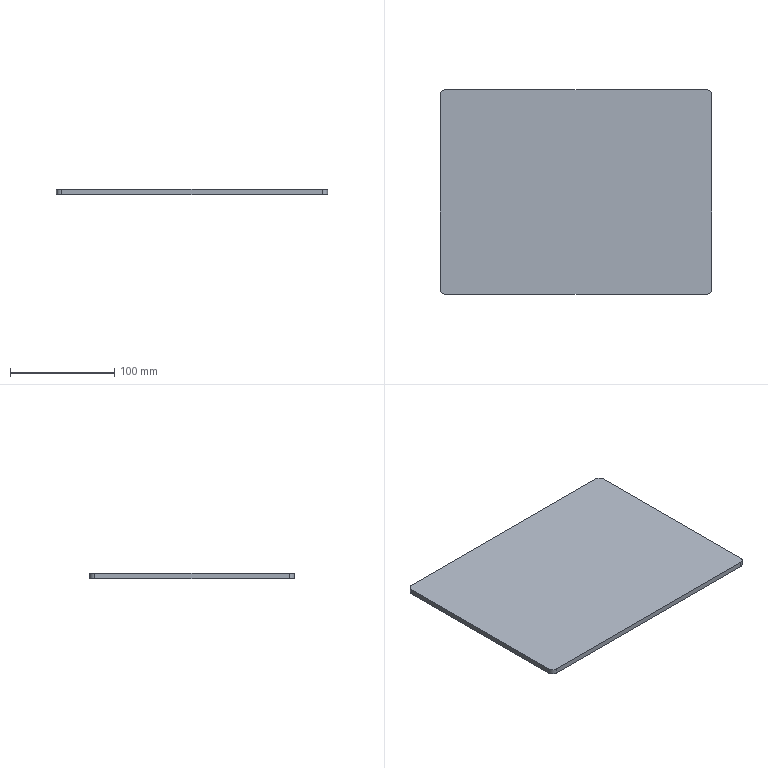Part | SolidWorks | features Extrusion 1, Fillet 1 | 1 solid | 10 faces | box 260 x 196 x 5 mm | volume 254693 mm3 | plane 6 | cylinder 4 | commonest cylinder face diameters 10 x4
STEP:
#1=CARTESIAN_POINT('',(0.,-5.,0.));
#2=VERTEX_POINT('',#1);
#3=CARTESIAN_POINT('',(0.,-191.,0.));
#4=VERTEX_POINT('',#3);
#5=CARTESIAN_POINT('',(0.,0.,0.));
#6=DIRECTION('',(0.,-1.,0.));
#7=VECTOR('',#6,1000.);
#8=LINE('',#5,#7);
#9=EDGE_CURVE('',#2,#4,#8,.T.);
#10=ORIENTED_EDGE('',*,*,#9,.T.);
#11=CARTESIAN_POINT('',(0.,-191.,5.));
#12=VERTEX_POINT('',#11);
#13=CARTESIAN_POINT('',(0.,-191.,5.));
#14=DIRECTION('',(0.,0.,1.));
#15=VECTOR('',#14,1000.);
#16=LINE('',#13,#15);
#17=EDGE_CURVE('',#4,#12,#16,.T.);
#18=ORIENTED_EDGE('',*,*,#17,.T.);
#19=CARTESIAN_POINT('',(0.,-5.,5.));
#20=VERTEX_POINT('',#19);
#21=CARTESIAN_POINT('',(0.,0.,5.));
#22=DIRECTION('',(0.,-1.,0.));
#23=VECTOR('',#22,1000.);
#24=LINE('',#21,#23);
#25=EDGE_CURVE('',#20,#12,#24,.T.);
#26=ORIENTED_EDGE('',*,*,#25,.F.);
#27=CARTESIAN_POINT('',(0.,-5.,5.));
#28=DIRECTION('',(0.,0.,-1.));
#29=VECTOR('',#28,1000.);
#30=LINE('',#27,#29);
#31=EDGE_CURVE('',#20,#2,#30,.T.);
#32=ORIENTED_EDGE('',*,*,#31,.T.);
#33=EDGE_LOOP('',(#10,#18,#26,#32));
#34=FACE_OUTER_BOUND('',#33,.T.);
#35=CARTESIAN_POINT('',(0.,0.,5.));
#36=DIRECTION('',(1.,0.,0.));
#37=DIRECTION('',(0.,1.,0.));
#38=AXIS2_PLACEMENT_3D('',#35,#36,#37);
#39=PLANE('',#38);
#40=ADVANCED_FACE('',(#34),#39,.F.);
#41=CARTESIAN_POINT('',(5.,-196.,0.));
#42=VERTEX_POINT('',#41);
#43=CARTESIAN_POINT('',(255.,-196.,0.));
#44=VERTEX_POINT('',#43);
#45=CARTESIAN_POINT('',(0.,-196.,0.));
#46=DIRECTION('',(1.,0.,0.));
#47=VECTOR('',#46,1000.);
#48=LINE('',#45,#47);
#49=EDGE_CURVE('',#42,#44,#48,.T.);
#50=ORIENTED_EDGE('',*,*,#49,.T.);
#51=CARTESIAN_POINT('',(255.,-196.,5.));
#52=VERTEX_POINT('',#51);
#53=CARTESIAN_POINT('',(255.,-196.,5.));
#54=DIRECTION('',(0.,0.,1.));
#55=VECTOR('',#54,1000.);
#56=LINE('',#53,#55);
#57=EDGE_CURVE('',#44,#52,#56,.T.);
#58=ORIENTED_EDGE('',*,*,#57,.T.);
#59=CARTESIAN_POINT('',(5.,-196.,5.));
#60=VERTEX_POINT('',#59);
#61=CARTESIAN_POINT('',(0.,-196.,5.));
#62=DIRECTION('',(1.,0.,0.));
#63=VECTOR('',#62,1000.);
#64=LINE('',#61,#63);
#65=EDGE_CURVE('',#60,#52,#64,.T.);
#66=ORIENTED_EDGE('',*,*,#65,.F.);
#67=CARTESIAN_POINT('',(5.,-196.,5.));
#68=DIRECTION('',(0.,0.,-1.));
#69=VECTOR('',#68,1000.);
#70=LINE('',#67,#69);
#71=EDGE_CURVE('',#60,#42,#70,.T.);
#72=ORIENTED_EDGE('',*,*,#71,.T.);
#73=EDGE_LOOP('',(#50,#58,#66,#72));
#74=FACE_OUTER_BOUND('',#73,.T.);
#75=CARTESIAN_POINT('',(0.,-196.,5.));
#76=DIRECTION('',(0.,1.,0.));
#77=DIRECTION('',(0.,0.,1.));
#78=AXIS2_PLACEMENT_3D('',#75,#76,#77);
#79=PLANE('',#78);
#80=ADVANCED_FACE('',(#74),#79,.F.);
#81=CARTESIAN_POINT('',(260.,-191.,0.));
#82=VERTEX_POINT('',#81);
#83=CARTESIAN_POINT('',(260.,-5.,0.));
#84=VERTEX_POINT('',#83);
#85=CARTESIAN_POINT('',(260.,0.,0.));
#86=DIRECTION('',(0.,1.,0.));
#87=VECTOR('',#86,1000.);
#88=LINE('',#85,#87);
#89=EDGE_CURVE('',#82,#84,#88,.T.);
#90=ORIENTED_EDGE('',*,*,#89,.T.);
#91=CARTESIAN_POINT('',(260.,-5.,5.));
#92=VERTEX_POINT('',#91);
#93=CARTESIAN_POINT('',(260.,-5.,5.));
#94=DIRECTION('',(0.,0.,1.));
#95=VECTOR('',#94,1000.);
#96=LINE('',#93,#95);
#97=EDGE_CURVE('',#84,#92,#96,.T.);
#98=ORIENTED_EDGE('',*,*,#97,.T.);
#99=CARTESIAN_POINT('',(260.,-191.,5.));
#100=VERTEX_POINT('',#99);
#101=CARTESIAN_POINT('',(260.,0.,5.));
#102=DIRECTION('',(0.,1.,0.));
#103=VECTOR('',#102,1000.);
#104=LINE('',#101,#103);
#105=EDGE_CURVE('',#100,#92,#104,.T.);
#106=ORIENTED_EDGE('',*,*,#105,.F.);
#107=CARTESIAN_POINT('',(260.,-191.,5.));
#108=DIRECTION('',(0.,0.,-1.));
#109=VECTOR('',#108,1000.);
#110=LINE('',#107,#109);
#111=EDGE_CURVE('',#100,#82,#110,.T.);
#112=ORIENTED_EDGE('',*,*,#111,.T.);
#113=EDGE_LOOP('',(#90,#98,#106,#112));
#114=FACE_OUTER_BOUND('',#113,.T.);
#115=CARTESIAN_POINT('',(260.,0.,5.));
#116=DIRECTION('',(-1.,0.,0.));
#117=DIRECTION('',(0.,0.,1.));
#118=AXIS2_PLACEMENT_3D('',#115,#116,#117);
#119=PLANE('',#118);
#120=ADVANCED_FACE('',(#114),#119,.F.);
#121=CARTESIAN_POINT('',(255.,0.,5.));
#122=VERTEX_POINT('',#121);
#123=CARTESIAN_POINT('',(5.,0.,5.));
#124=VERTEX_POINT('',#123);
#125=CARTESIAN_POINT('',(0.,0.,5.));
#126=DIRECTION('',(-1.,0.,0.));
#127=VECTOR('',#126,1000.);
#128=LINE('',#125,#127);
#129=EDGE_CURVE('',#122,#124,#128,.T.);
#130=ORIENTED_EDGE('',*,*,#129,.F.);
#131=CARTESIAN_POINT('',(255.,0.,0.));
#132=VERTEX_POINT('',#131);
#133=CARTESIAN_POINT('',(255.,0.,5.));
#134=DIRECTION('',(0.,0.,-1.));
#135=VECTOR('',#134,1000.);
#136=LINE('',#133,#135);
#137=EDGE_CURVE('',#122,#132,#136,.T.);
#138=ORIENTED_EDGE('',*,*,#137,.T.);
#139=CARTESIAN_POINT('',(5.,0.,0.));
#140=VERTEX_POINT('',#139);
#141=CARTESIAN_POINT('',(0.,0.,0.));
#142=DIRECTION('',(-1.,0.,0.));
#143=VECTOR('',#142,1000.);
#144=LINE('',#141,#143);
#145=EDGE_CURVE('',#132,#140,#144,.T.);
#146=ORIENTED_EDGE('',*,*,#145,.T.);
#147=CARTESIAN_POINT('',(5.,0.,5.));
#148=DIRECTION('',(0.,0.,1.));
#149=VECTOR('',#148,1000.);
#150=LINE('',#147,#149);
#151=EDGE_CURVE('',#140,#124,#150,.T.);
#152=ORIENTED_EDGE('',*,*,#151,.T.);
#153=EDGE_LOOP('',(#130,#138,#146,#152));
#154=FACE_OUTER_BOUND('',#153,.T.);
#155=CARTESIAN_POINT('',(0.,0.,5.));
#156=DIRECTION('',(0.,-1.,0.));
#157=DIRECTION('',(0.,0.,-1.));
#158=AXIS2_PLACEMENT_3D('',#155,#156,#157);
#159=PLANE('',#158);
#160=ADVANCED_FACE('',(#154),#159,.F.);
#161=ORIENTED_EDGE('',*,*,#105,.T.);
#162=CARTESIAN_POINT('',(255.,-5.,5.));
#163=DIRECTION('',(0.,0.,1.));
#164=DIRECTION('',(1.,0.,0.));
#165=AXIS2_PLACEMENT_3D('',#162,#163,#164);
#166=CIRCLE('',#165,5.);
#167=EDGE_CURVE('',#92,#122,#166,.T.);
#168=ORIENTED_EDGE('',*,*,#167,.T.);
#169=ORIENTED_EDGE('',*,*,#129,.T.);
#170=CARTESIAN_POINT('',(5.,-5.,5.));
#171=DIRECTION('',(0.,0.,1.));
#172=DIRECTION('',(1.,0.,0.));
#173=AXIS2_PLACEMENT_3D('',#170,#171,#172);
#174=CIRCLE('',#173,5.);
#175=EDGE_CURVE('',#124,#20,#174,.T.);
#176=ORIENTED_EDGE('',*,*,#175,.T.);
#177=ORIENTED_EDGE('',*,*,#25,.T.);
#178=CARTESIAN_POINT('',(5.,-191.,5.));
#179=DIRECTION('',(0.,0.,1.));
#180=DIRECTION('',(1.,0.,0.));
#181=AXIS2_PLACEMENT_3D('',#178,#179,#180);
#182=CIRCLE('',#181,5.);
#183=EDGE_CURVE('',#12,#60,#182,.T.);
#184=ORIENTED_EDGE('',*,*,#183,.T.);
#185=ORIENTED_EDGE('',*,*,#65,.T.);
#186=CARTESIAN_POINT('',(255.,-191.,5.));
#187=DIRECTION('',(0.,0.,1.));
#188=DIRECTION('',(1.,0.,0.));
#189=AXIS2_PLACEMENT_3D('',#186,#187,#188);
#190=CIRCLE('',#189,5.);
#191=EDGE_CURVE('',#52,#100,#190,.T.);
#192=ORIENTED_EDGE('',*,*,#191,.T.);
#193=EDGE_LOOP('',(#161,#168,#169,#176,#177,#184,#185,#192));
#194=FACE_OUTER_BOUND('',#193,.T.);
#195=CARTESIAN_POINT('',(0.,0.,5.));
#196=DIRECTION('',(0.,0.,1.));
#197=DIRECTION('',(1.,0.,0.));
#198=AXIS2_PLACEMENT_3D('',#195,#196,#197);
#199=PLANE('',#198);
#200=ADVANCED_FACE('',(#194),#199,.T.);
#201=ORIENTED_EDGE('',*,*,#145,.F.);
#202=CARTESIAN_POINT('',(255.,-5.,0.));
#203=DIRECTION('',(0.,0.,-1.));
#204=DIRECTION('',(1.,0.,0.));
#205=AXIS2_PLACEMENT_3D('',#202,#203,#204);
#206=CIRCLE('',#205,5.);
#207=EDGE_CURVE('',#132,#84,#206,.T.);
#208=ORIENTED_EDGE('',*,*,#207,.T.);
#209=ORIENTED_EDGE('',*,*,#89,.F.);
#210=CARTESIAN_POINT('',(255.,-191.,0.));
#211=DIRECTION('',(0.,0.,-1.));
#212=DIRECTION('',(1.,0.,0.));
#213=AXIS2_PLACEMENT_3D('',#210,#211,#212);
#214=CIRCLE('',#213,5.);
#215=EDGE_CURVE('',#82,#44,#214,.T.);
#216=ORIENTED_EDGE('',*,*,#215,.T.);
#217=ORIENTED_EDGE('',*,*,#49,.F.);
#218=CARTESIAN_POINT('',(5.,-191.,0.));
#219=DIRECTION('',(0.,0.,-1.));
#220=DIRECTION('',(1.,0.,0.));
#221=AXIS2_PLACEMENT_3D('',#218,#219,#220);
#222=CIRCLE('',#221,5.);
#223=EDGE_CURVE('',#42,#4,#222,.T.);
#224=ORIENTED_EDGE('',*,*,#223,.T.);
#225=ORIENTED_EDGE('',*,*,#9,.F.);
#226=CARTESIAN_POINT('',(5.,-5.,0.));
#227=DIRECTION('',(0.,0.,-1.));
#228=DIRECTION('',(1.,0.,0.));
#229=AXIS2_PLACEMENT_3D('',#226,#227,#228);
#230=CIRCLE('',#229,5.);
#231=EDGE_CURVE('',#2,#140,#230,.T.);
#232=ORIENTED_EDGE('',*,*,#231,.T.);
#233=EDGE_LOOP('',(#201,#208,#209,#216,#217,#224,#225,#232));
#234=FACE_OUTER_BOUND('',#233,.T.);
#235=CARTESIAN_POINT('',(0.,0.,0.));
#236=DIRECTION('',(0.,0.,1.));
#237=DIRECTION('',(1.,0.,0.));
#238=AXIS2_PLACEMENT_3D('',#235,#236,#237);
#239=PLANE('',#238);
#240=ADVANCED_FACE('',(#234),#239,.F.);
#241=ORIENTED_EDGE('',*,*,#167,.F.);
#242=ORIENTED_EDGE('',*,*,#97,.F.);
#243=ORIENTED_EDGE('',*,*,#207,.F.);
#244=ORIENTED_EDGE('',*,*,#137,.F.);
#245=EDGE_LOOP('',(#241,#242,#243,#244));
#246=FACE_OUTER_BOUND('',#245,.T.);
#247=CARTESIAN_POINT('',(255.,-5.,5.));
#248=DIRECTION('',(0.,0.,-1.));
#249=DIRECTION('',(-1.,0.,0.));
#250=AXIS2_PLACEMENT_3D('',#247,#248,#249);
#251=CYLINDRICAL_SURFACE('',#250,5.);
#252=ADVANCED_FACE('',(#246),#251,.T.);
#253=ORIENTED_EDGE('',*,*,#191,.F.);
#254=ORIENTED_EDGE('',*,*,#57,.F.);
#255=ORIENTED_EDGE('',*,*,#215,.F.);
#256=ORIENTED_EDGE('',*,*,#111,.F.);
#257=EDGE_LOOP('',(#253,#254,#255,#256));
#258=FACE_OUTER_BOUND('',#257,.T.);
#259=CARTESIAN_POINT('',(255.,-191.,5.));
#260=DIRECTION('',(0.,0.,-1.));
#261=DIRECTION('',(-1.,0.,0.));
#262=AXIS2_PLACEMENT_3D('',#259,#260,#261);
#263=CYLINDRICAL_SURFACE('',#262,5.);
#264=ADVANCED_FACE('',(#258),#263,.T.);
#265=ORIENTED_EDGE('',*,*,#183,.F.);
#266=ORIENTED_EDGE('',*,*,#17,.F.);
#267=ORIENTED_EDGE('',*,*,#223,.F.);
#268=ORIENTED_EDGE('',*,*,#71,.F.);
#269=EDGE_LOOP('',(#265,#266,#267,#268));
#270=FACE_OUTER_BOUND('',#269,.T.);
#271=CARTESIAN_POINT('',(5.,-191.,5.));
#272=DIRECTION('',(0.,0.,-1.));
#273=DIRECTION('',(-1.,0.,0.));
#274=AXIS2_PLACEMENT_3D('',#271,#272,#273);
#275=CYLINDRICAL_SURFACE('',#274,5.);
#276=ADVANCED_FACE('',(#270),#275,.T.);
#277=ORIENTED_EDGE('',*,*,#175,.F.);
#278=ORIENTED_EDGE('',*,*,#151,.F.);
#279=ORIENTED_EDGE('',*,*,#231,.F.);
#280=ORIENTED_EDGE('',*,*,#31,.F.);
#281=EDGE_LOOP('',(#277,#278,#279,#280));
#282=FACE_OUTER_BOUND('',#281,.T.);
#283=CARTESIAN_POINT('',(5.,-5.,5.));
#284=DIRECTION('',(0.,0.,-1.));
#285=DIRECTION('',(-1.,0.,0.));
#286=AXIS2_PLACEMENT_3D('',#283,#284,#285);
#287=CYLINDRICAL_SURFACE('',#286,5.);
#288=ADVANCED_FACE('',(#282),#287,.T.);
#289=CLOSED_SHELL('',(#40,#80,#120,#160,#200,#240,#252,#264,#276,#288));
#290=MANIFOLD_SOLID_BREP('',#289);
#291=CARTESIAN_POINT('',(0.,0.,0.));
#292=DIRECTION('',(0.,0.,1.));
#293=DIRECTION('',(1.,0.,0.));
#294=AXIS2_PLACEMENT_3D('',#291,#292,#293);
#295=(LENGTH_UNIT()NAMED_UNIT(*)SI_UNIT(.MILLI.,.METRE.));
#296=UNCERTAINTY_MEASURE_WITH_UNIT(LENGTH_MEASURE(0.00001),#295,'','');
#297=(NAMED_UNIT(*)PLANE_ANGLE_UNIT()SI_UNIT($,.RADIAN.));
#298=(NAMED_UNIT(*)SI_UNIT($,.STERADIAN.)SOLID_ANGLE_UNIT());
#299=(GEOMETRIC_REPRESENTATION_CONTEXT(3)GLOBAL_UNCERTAINTY_ASSIGNED_CONTEXT((#296))GLOBAL_UNIT_ASSIGNED_CONTEXT((#295,#297,#298))REPRESENTATION_CONTEXT('',''));
#300=ADVANCED_BREP_SHAPE_REPRESENTATION('',(#290,#294),#299);